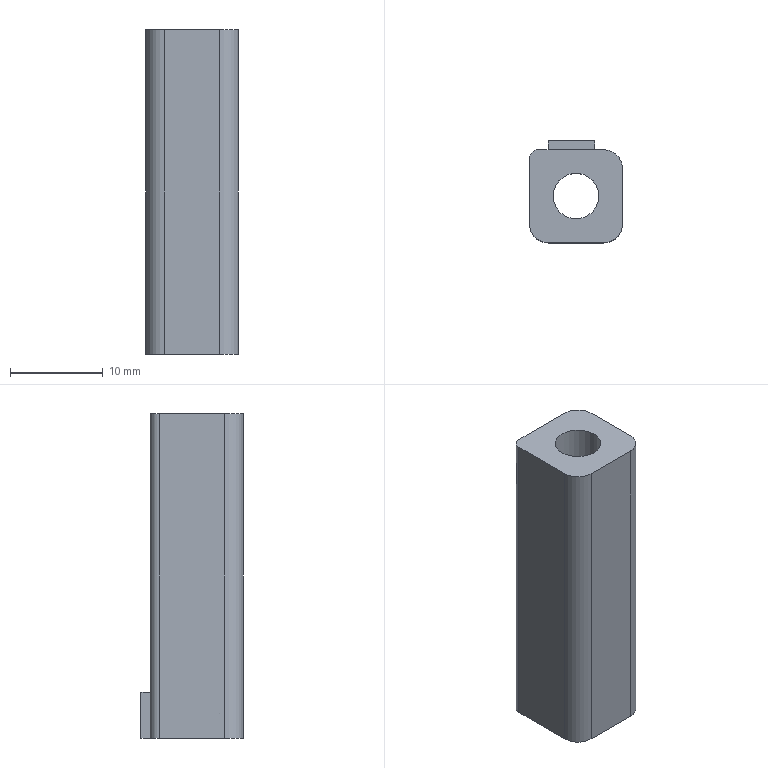Part | NX | features DIE-91 2 | 1 solid | 17 faces | box 10 x 11 x 35 mm | volume 2507 mm3 | plane 11 | cylinder 6 | commonest cylinder face diameters 4 x3 2 x1 4.92 x1 5.92 x1
STEP:
#1=CARTESIAN_POINT('',(4108.236,-844.622,828.716));
#2=VERTEX_POINT('',#1);
#3=CARTESIAN_POINT('',(4113.236,-844.622,828.716));
#4=VERTEX_POINT('',#3);
#5=CARTESIAN_POINT('',(4111.236,-844.622,828.716));
#6=DIRECTION('',(1.,0.,0.));
#7=VECTOR('',#6,1000.);
#8=LINE('',#5,#7);
#9=EDGE_CURVE('',#2,#4,#8,.T.);
#10=ORIENTED_EDGE('',*,*,#9,.F.);
#11=CARTESIAN_POINT('',(4108.236,-844.622,823.716));
#12=VERTEX_POINT('',#11);
#13=CARTESIAN_POINT('',(4108.236,-844.622,823.716));
#14=DIRECTION('',(0.,0.,-1.));
#15=VECTOR('',#14,1000.);
#16=LINE('',#13,#15);
#17=EDGE_CURVE('',#2,#12,#16,.T.);
#18=ORIENTED_EDGE('',*,*,#17,.T.);
#19=CARTESIAN_POINT('',(4107.236,-844.622,823.716));
#20=VERTEX_POINT('',#19);
#21=CARTESIAN_POINT('',(4111.236,-844.622,823.716));
#22=DIRECTION('',(-1.,0.,0.));
#23=VECTOR('',#22,1000.);
#24=LINE('',#21,#23);
#25=EDGE_CURVE('',#20,#12,#24,.F.);
#26=ORIENTED_EDGE('',*,*,#25,.F.);
#27=CARTESIAN_POINT('',(4107.236,-844.622,858.716));
#28=VERTEX_POINT('',#27);
#29=CARTESIAN_POINT('',(4107.236,-844.622,823.716));
#30=DIRECTION('',(0.,0.,1.));
#31=VECTOR('',#30,1000.);
#32=LINE('',#29,#31);
#33=EDGE_CURVE('',#20,#28,#32,.T.);
#34=ORIENTED_EDGE('',*,*,#33,.T.);
#35=CARTESIAN_POINT('',(4114.236,-844.622,858.716));
#36=VERTEX_POINT('',#35);
#37=CARTESIAN_POINT('',(4111.236,-844.622,858.716));
#38=DIRECTION('',(1.,0.,0.));
#39=VECTOR('',#38,1000.);
#40=LINE('',#37,#39);
#41=EDGE_CURVE('',#28,#36,#40,.T.);
#42=ORIENTED_EDGE('',*,*,#41,.T.);
#43=CARTESIAN_POINT('',(4114.236,-844.622,823.716));
#44=VERTEX_POINT('',#43);
#45=CARTESIAN_POINT('',(4114.236,-844.622,823.716));
#46=DIRECTION('',(0.,0.,1.));
#47=VECTOR('',#46,1000.);
#48=LINE('',#45,#47);
#49=EDGE_CURVE('',#36,#44,#48,.F.);
#50=ORIENTED_EDGE('',*,*,#49,.T.);
#51=CARTESIAN_POINT('',(4113.236,-844.622,823.716));
#52=VERTEX_POINT('',#51);
#53=CARTESIAN_POINT('',(4111.236,-844.622,823.716));
#54=DIRECTION('',(-1.,0.,0.));
#55=VECTOR('',#54,1000.);
#56=LINE('',#53,#55);
#57=EDGE_CURVE('',#52,#44,#56,.F.);
#58=ORIENTED_EDGE('',*,*,#57,.F.);
#59=CARTESIAN_POINT('',(4113.236,-844.622,823.716));
#60=DIRECTION('',(0.,0.,1.));
#61=VECTOR('',#60,1000.);
#62=LINE('',#59,#61);
#63=EDGE_CURVE('',#52,#4,#62,.T.);
#64=ORIENTED_EDGE('',*,*,#63,.T.);
#65=EDGE_LOOP('',(#10,#18,#26,#34,#42,#50,#58,#64));
#66=FACE_BOUND('',#65,.T.);
#67=CARTESIAN_POINT('',(4111.236,-844.622,823.716));
#68=DIRECTION('',(0.,1.,0.));
#69=DIRECTION('',(0.,0.,1.));
#70=AXIS2_PLACEMENT_3D('',#67,#68,#69);
#71=PLANE('',#70);
#72=ADVANCED_FACE('',(#66),#71,.T.);
#73=CARTESIAN_POINT('',(4108.276,-849.622,823.716));
#74=VERTEX_POINT('',#73);
#75=CARTESIAN_POINT('',(4111.236,-849.622,823.716));
#76=DIRECTION('',(0.,0.,-1.));
#77=DIRECTION('',(-1.,0.,0.));
#78=AXIS2_PLACEMENT_3D('',#75,#76,#77);
#79=CIRCLE('',#78,2.96);
#80=EDGE_CURVE('',#74,#74,#79,.T.);
#81=ORIENTED_EDGE('',*,*,#80,.T.);
#82=CARTESIAN_POINT('',(4108.276,-849.622,853.716));
#83=VERTEX_POINT('',#82);
#84=CARTESIAN_POINT('',(4108.276,-849.622,862.216));
#85=DIRECTION('',(0.,0.,-1.));
#86=VECTOR('',#85,1000.);
#87=LINE('',#84,#86);
#88=EDGE_CURVE('',#83,#74,#87,.T.);
#89=ORIENTED_EDGE('',*,*,#88,.F.);
#90=CARTESIAN_POINT('',(4111.236,-849.622,853.716));
#91=DIRECTION('',(0.,0.,1.));
#92=DIRECTION('',(1.,0.,0.));
#93=AXIS2_PLACEMENT_3D('',#90,#91,#92);
#94=CIRCLE('',#93,2.96);
#95=EDGE_CURVE('',#83,#83,#94,.F.);
#96=ORIENTED_EDGE('',*,*,#95,.F.);
#97=ORIENTED_EDGE('',*,*,#88,.T.);
#98=EDGE_LOOP('',(#81,#89,#96,#97));
#99=FACE_BOUND('',#98,.T.);
#100=CARTESIAN_POINT('',(4111.236,-849.622,862.216));
#101=DIRECTION('',(0.,0.,-1.));
#102=DIRECTION('',(-1.,0.,0.));
#103=AXIS2_PLACEMENT_3D('',#100,#101,#102);
#104=CYLINDRICAL_SURFACE('',#103,2.96);
#105=ADVANCED_FACE('',(#99),#104,.F.);
#106=ORIENTED_EDGE('',*,*,#25,.T.);
#107=CARTESIAN_POINT('',(4108.236,-843.622,823.716));
#108=VERTEX_POINT('',#107);
#109=CARTESIAN_POINT('',(4108.236,-843.622,823.716));
#110=DIRECTION('',(0.,-1.,0.));
#111=VECTOR('',#110,1000.);
#112=LINE('',#109,#111);
#113=EDGE_CURVE('',#108,#12,#112,.T.);
#114=ORIENTED_EDGE('',*,*,#113,.F.);
#115=CARTESIAN_POINT('',(4113.236,-843.622,823.716));
#116=VERTEX_POINT('',#115);
#117=CARTESIAN_POINT('',(4114.236,-843.622,823.716));
#118=DIRECTION('',(-1.,0.,0.));
#119=VECTOR('',#118,1000.);
#120=LINE('',#117,#119);
#121=EDGE_CURVE('',#116,#108,#120,.T.);
#122=ORIENTED_EDGE('',*,*,#121,.F.);
#123=CARTESIAN_POINT('',(4113.236,-844.672,823.716));
#124=DIRECTION('',(0.,1.,0.));
#125=VECTOR('',#124,1000.);
#126=LINE('',#123,#125);
#127=EDGE_CURVE('',#52,#116,#126,.T.);
#128=ORIENTED_EDGE('',*,*,#127,.F.);
#129=ORIENTED_EDGE('',*,*,#57,.T.);
#130=CARTESIAN_POINT('',(4116.236,-846.622,823.716));
#131=VERTEX_POINT('',#130);
#132=CARTESIAN_POINT('',(4114.236,-846.622,823.716));
#133=DIRECTION('',(0.,0.,-1.));
#134=DIRECTION('',(-1.,0.,0.));
#135=AXIS2_PLACEMENT_3D('',#132,#133,#134);
#136=CIRCLE('',#135,2.);
#137=EDGE_CURVE('',#131,#44,#136,.F.);
#138=ORIENTED_EDGE('',*,*,#137,.F.);
#139=CARTESIAN_POINT('',(4116.236,-852.622,823.716));
#140=VERTEX_POINT('',#139);
#141=CARTESIAN_POINT('',(4116.236,-849.622,823.716));
#142=DIRECTION('',(0.,1.,0.));
#143=VECTOR('',#142,1000.);
#144=LINE('',#141,#143);
#145=EDGE_CURVE('',#140,#131,#144,.T.);
#146=ORIENTED_EDGE('',*,*,#145,.F.);
#147=CARTESIAN_POINT('',(4114.236,-854.622,823.716));
#148=VERTEX_POINT('',#147);
#149=CARTESIAN_POINT('',(4114.236,-852.622,823.716));
#150=DIRECTION('',(0.,0.,-1.));
#151=DIRECTION('',(-1.,0.,0.));
#152=AXIS2_PLACEMENT_3D('',#149,#150,#151);
#153=CIRCLE('',#152,2.);
#154=EDGE_CURVE('',#140,#148,#153,.T.);
#155=ORIENTED_EDGE('',*,*,#154,.T.);
#156=CARTESIAN_POINT('',(4108.236,-854.622,823.716));
#157=VERTEX_POINT('',#156);
#158=CARTESIAN_POINT('',(4111.236,-854.622,823.716));
#159=DIRECTION('',(1.,0.,0.));
#160=VECTOR('',#159,1000.);
#161=LINE('',#158,#160);
#162=EDGE_CURVE('',#157,#148,#161,.T.);
#163=ORIENTED_EDGE('',*,*,#162,.F.);
#164=CARTESIAN_POINT('',(4106.236,-852.622,823.716));
#165=VERTEX_POINT('',#164);
#166=CARTESIAN_POINT('',(4108.236,-852.622,823.716));
#167=DIRECTION('',(0.,0.,-1.));
#168=DIRECTION('',(-1.,0.,0.));
#169=AXIS2_PLACEMENT_3D('',#166,#167,#168);
#170=CIRCLE('',#169,2.);
#171=EDGE_CURVE('',#157,#165,#170,.T.);
#172=ORIENTED_EDGE('',*,*,#171,.T.);
#173=CARTESIAN_POINT('',(4106.236,-845.622,823.716));
#174=VERTEX_POINT('',#173);
#175=CARTESIAN_POINT('',(4106.236,-849.622,823.716));
#176=DIRECTION('',(0.,-1.,0.));
#177=VECTOR('',#176,1000.);
#178=LINE('',#175,#177);
#179=EDGE_CURVE('',#165,#174,#178,.F.);
#180=ORIENTED_EDGE('',*,*,#179,.T.);
#181=CARTESIAN_POINT('',(4107.236,-845.622,823.716));
#182=DIRECTION('',(0.,0.,-1.));
#183=DIRECTION('',(-1.,0.,0.));
#184=AXIS2_PLACEMENT_3D('',#181,#182,#183);
#185=CIRCLE('',#184,1.);
#186=EDGE_CURVE('',#174,#20,#185,.T.);
#187=ORIENTED_EDGE('',*,*,#186,.T.);
#188=EDGE_LOOP('',(#106,#114,#122,#128,#129,#138,#146,#155,#163,#172,#180,#187));
#189=FACE_BOUND('',#188,.T.);
#190=ORIENTED_EDGE('',*,*,#80,.F.);
#191=EDGE_LOOP('',(#190));
#192=FACE_BOUND('',#191,.T.);
#193=CARTESIAN_POINT('',(4123.586,-858.122,823.716));
#194=DIRECTION('',(0.,0.,-1.));
#195=DIRECTION('',(-1.,0.,0.));
#196=AXIS2_PLACEMENT_3D('',#193,#194,#195);
#197=PLANE('',#196);
#198=ADVANCED_FACE('',(#189,#192),#197,.T.);
#199=CARTESIAN_POINT('',(4108.776,-849.622,853.716));
#200=VERTEX_POINT('',#199);
#201=CARTESIAN_POINT('',(4111.236,-849.622,853.716));
#202=DIRECTION('',(0.,0.,1.));
#203=DIRECTION('',(1.,0.,0.));
#204=AXIS2_PLACEMENT_3D('',#201,#202,#203);
#205=CIRCLE('',#204,2.46);
#206=EDGE_CURVE('',#200,#200,#205,.T.);
#207=ORIENTED_EDGE('',*,*,#206,.T.);
#208=EDGE_LOOP('',(#207));
#209=FACE_BOUND('',#208,.T.);
#210=ORIENTED_EDGE('',*,*,#95,.T.);
#211=EDGE_LOOP('',(#210));
#212=FACE_BOUND('',#211,.T.);
#213=CARTESIAN_POINT('',(4079.736,-858.122,853.716));
#214=DIRECTION('',(0.,0.,1.));
#215=DIRECTION('',(1.,0.,0.));
#216=AXIS2_PLACEMENT_3D('',#213,#214,#215);
#217=PLANE('',#216);
#218=ADVANCED_FACE('',(#209,#212),#217,.F.);
#219=CARTESIAN_POINT('',(4108.776,-849.622,858.716));
#220=VERTEX_POINT('',#219);
#221=CARTESIAN_POINT('',(4108.776,-849.622,862.216));
#222=DIRECTION('',(0.,0.,-1.));
#223=VECTOR('',#222,1000.);
#224=LINE('',#221,#223);
#225=EDGE_CURVE('',#220,#200,#224,.T.);
#226=ORIENTED_EDGE('',*,*,#225,.T.);
#227=ORIENTED_EDGE('',*,*,#206,.F.);
#228=ORIENTED_EDGE('',*,*,#225,.F.);
#229=CARTESIAN_POINT('',(4111.236,-849.622,858.716));
#230=DIRECTION('',(0.,0.,1.));
#231=DIRECTION('',(1.,0.,0.));
#232=AXIS2_PLACEMENT_3D('',#229,#230,#231);
#233=CIRCLE('',#232,2.46);
#234=EDGE_CURVE('',#220,#220,#233,.T.);
#235=ORIENTED_EDGE('',*,*,#234,.T.);
#236=EDGE_LOOP('',(#226,#227,#228,#235));
#237=FACE_BOUND('',#236,.T.);
#238=CARTESIAN_POINT('',(4111.236,-849.622,862.216));
#239=DIRECTION('',(0.,0.,-1.));
#240=DIRECTION('',(-1.,0.,0.));
#241=AXIS2_PLACEMENT_3D('',#238,#239,#240);
#242=CYLINDRICAL_SURFACE('',#241,2.46);
#243=ADVANCED_FACE('',(#237),#242,.F.);
#244=ORIENTED_EDGE('',*,*,#234,.F.);
#245=EDGE_LOOP('',(#244));
#246=FACE_BOUND('',#245,.T.);
#247=CARTESIAN_POINT('',(4106.236,-852.622,858.716));
#248=VERTEX_POINT('',#247);
#249=CARTESIAN_POINT('',(4106.236,-845.622,858.716));
#250=VERTEX_POINT('',#249);
#251=CARTESIAN_POINT('',(4106.236,-849.622,858.716));
#252=DIRECTION('',(0.,1.,0.));
#253=VECTOR('',#252,1000.);
#254=LINE('',#251,#253);
#255=EDGE_CURVE('',#248,#250,#254,.T.);
#256=ORIENTED_EDGE('',*,*,#255,.F.);
#257=CARTESIAN_POINT('',(4108.236,-854.622,858.716));
#258=VERTEX_POINT('',#257);
#259=CARTESIAN_POINT('',(4108.236,-852.622,858.716));
#260=DIRECTION('',(0.,0.,1.));
#261=DIRECTION('',(1.,0.,0.));
#262=AXIS2_PLACEMENT_3D('',#259,#260,#261);
#263=CIRCLE('',#262,2.);
#264=EDGE_CURVE('',#258,#248,#263,.F.);
#265=ORIENTED_EDGE('',*,*,#264,.F.);
#266=CARTESIAN_POINT('',(4114.236,-854.622,858.716));
#267=VERTEX_POINT('',#266);
#268=CARTESIAN_POINT('',(4111.236,-854.622,858.716));
#269=DIRECTION('',(-1.,0.,0.));
#270=VECTOR('',#269,1000.);
#271=LINE('',#268,#270);
#272=EDGE_CURVE('',#258,#267,#271,.F.);
#273=ORIENTED_EDGE('',*,*,#272,.T.);
#274=CARTESIAN_POINT('',(4116.236,-852.622,858.716));
#275=VERTEX_POINT('',#274);
#276=CARTESIAN_POINT('',(4114.236,-852.622,858.716));
#277=DIRECTION('',(0.,0.,1.));
#278=DIRECTION('',(1.,0.,0.));
#279=AXIS2_PLACEMENT_3D('',#276,#277,#278);
#280=CIRCLE('',#279,2.);
#281=EDGE_CURVE('',#275,#267,#280,.F.);
#282=ORIENTED_EDGE('',*,*,#281,.F.);
#283=CARTESIAN_POINT('',(4116.236,-846.622,858.716));
#284=VERTEX_POINT('',#283);
#285=CARTESIAN_POINT('',(4116.236,-849.622,858.716));
#286=DIRECTION('',(0.,-1.,0.));
#287=VECTOR('',#286,1000.);
#288=LINE('',#285,#287);
#289=EDGE_CURVE('',#275,#284,#288,.F.);
#290=ORIENTED_EDGE('',*,*,#289,.T.);
#291=CARTESIAN_POINT('',(4114.236,-846.622,858.716));
#292=DIRECTION('',(0.,0.,1.));
#293=DIRECTION('',(1.,0.,0.));
#294=AXIS2_PLACEMENT_3D('',#291,#292,#293);
#295=CIRCLE('',#294,2.);
#296=EDGE_CURVE('',#284,#36,#295,.T.);
#297=ORIENTED_EDGE('',*,*,#296,.T.);
#298=ORIENTED_EDGE('',*,*,#41,.F.);
#299=CARTESIAN_POINT('',(4107.236,-845.622,858.716));
#300=DIRECTION('',(0.,0.,1.));
#301=DIRECTION('',(1.,0.,0.));
#302=AXIS2_PLACEMENT_3D('',#299,#300,#301);
#303=CIRCLE('',#302,1.);
#304=EDGE_CURVE('',#28,#250,#303,.T.);
#305=ORIENTED_EDGE('',*,*,#304,.T.);
#306=EDGE_LOOP('',(#256,#265,#273,#282,#290,#297,#298,#305));
#307=FACE_BOUND('',#306,.T.);
#308=CARTESIAN_POINT('',(4123.586,-858.122,858.716));
#309=DIRECTION('',(0.,0.,1.));
#310=DIRECTION('',(-1.,0.,0.));
#311=AXIS2_PLACEMENT_3D('',#308,#309,#310);
#312=PLANE('',#311);
#313=ADVANCED_FACE('',(#246,#307),#312,.T.);
#314=ORIENTED_EDGE('',*,*,#186,.F.);
#315=CARTESIAN_POINT('',(4106.236,-845.622,823.716));
#316=DIRECTION('',(0.,0.,1.));
#317=VECTOR('',#316,1000.);
#318=LINE('',#315,#317);
#319=EDGE_CURVE('',#250,#174,#318,.F.);
#320=ORIENTED_EDGE('',*,*,#319,.F.);
#321=ORIENTED_EDGE('',*,*,#304,.F.);
#322=ORIENTED_EDGE('',*,*,#33,.F.);
#323=EDGE_LOOP('',(#314,#320,#321,#322));
#324=FACE_BOUND('',#323,.T.);
#325=CARTESIAN_POINT('',(4107.236,-845.622,823.716));
#326=DIRECTION('',(0.,0.,1.));
#327=DIRECTION('',(1.,0.,0.));
#328=AXIS2_PLACEMENT_3D('',#325,#326,#327);
#329=CYLINDRICAL_SURFACE('',#328,1.);
#330=ADVANCED_FACE('',(#324),#329,.T.);
#331=ORIENTED_EDGE('',*,*,#171,.F.);
#332=CARTESIAN_POINT('',(4108.236,-854.622,823.716));
#333=DIRECTION('',(0.,0.,1.));
#334=VECTOR('',#333,1000.);
#335=LINE('',#332,#334);
#336=EDGE_CURVE('',#258,#157,#335,.F.);
#337=ORIENTED_EDGE('',*,*,#336,.F.);
#338=ORIENTED_EDGE('',*,*,#264,.T.);
#339=CARTESIAN_POINT('',(4106.236,-852.622,823.716));
#340=DIRECTION('',(0.,0.,1.));
#341=VECTOR('',#340,1000.);
#342=LINE('',#339,#341);
#343=EDGE_CURVE('',#165,#248,#342,.T.);
#344=ORIENTED_EDGE('',*,*,#343,.F.);
#345=EDGE_LOOP('',(#331,#337,#338,#344));
#346=FACE_BOUND('',#345,.T.);
#347=CARTESIAN_POINT('',(4108.236,-852.622,823.716));
#348=DIRECTION('',(0.,0.,1.));
#349=DIRECTION('',(1.,0.,0.));
#350=AXIS2_PLACEMENT_3D('',#347,#348,#349);
#351=CYLINDRICAL_SURFACE('',#350,2.);
#352=ADVANCED_FACE('',(#346),#351,.T.);
#353=ORIENTED_EDGE('',*,*,#154,.F.);
#354=CARTESIAN_POINT('',(4116.236,-852.622,823.716));
#355=DIRECTION('',(0.,0.,1.));
#356=VECTOR('',#355,1000.);
#357=LINE('',#354,#356);
#358=EDGE_CURVE('',#275,#140,#357,.F.);
#359=ORIENTED_EDGE('',*,*,#358,.F.);
#360=ORIENTED_EDGE('',*,*,#281,.T.);
#361=CARTESIAN_POINT('',(4114.236,-854.622,823.716));
#362=DIRECTION('',(0.,0.,1.));
#363=VECTOR('',#362,1000.);
#364=LINE('',#361,#363);
#365=EDGE_CURVE('',#148,#267,#364,.T.);
#366=ORIENTED_EDGE('',*,*,#365,.F.);
#367=EDGE_LOOP('',(#353,#359,#360,#366));
#368=FACE_BOUND('',#367,.T.);
#369=CARTESIAN_POINT('',(4114.236,-852.622,823.716));
#370=DIRECTION('',(0.,0.,1.));
#371=DIRECTION('',(1.,0.,0.));
#372=AXIS2_PLACEMENT_3D('',#369,#370,#371);
#373=CYLINDRICAL_SURFACE('',#372,2.);
#374=ADVANCED_FACE('',(#368),#373,.T.);
#375=ORIENTED_EDGE('',*,*,#137,.T.);
#376=ORIENTED_EDGE('',*,*,#49,.F.);
#377=ORIENTED_EDGE('',*,*,#296,.F.);
#378=CARTESIAN_POINT('',(4116.236,-846.622,823.716));
#379=DIRECTION('',(0.,0.,1.));
#380=VECTOR('',#379,1000.);
#381=LINE('',#378,#380);
#382=EDGE_CURVE('',#131,#284,#381,.T.);
#383=ORIENTED_EDGE('',*,*,#382,.F.);
#384=EDGE_LOOP('',(#375,#376,#377,#383));
#385=FACE_BOUND('',#384,.T.);
#386=CARTESIAN_POINT('',(4114.236,-846.622,823.716));
#387=DIRECTION('',(0.,0.,1.));
#388=DIRECTION('',(1.,0.,0.));
#389=AXIS2_PLACEMENT_3D('',#386,#387,#388);
#390=CYLINDRICAL_SURFACE('',#389,2.);
#391=ADVANCED_FACE('',(#385),#390,.T.);
#392=ORIENTED_EDGE('',*,*,#145,.T.);
#393=ORIENTED_EDGE('',*,*,#382,.T.);
#394=ORIENTED_EDGE('',*,*,#289,.F.);
#395=ORIENTED_EDGE('',*,*,#358,.T.);
#396=EDGE_LOOP('',(#392,#393,#394,#395));
#397=FACE_BOUND('',#396,.T.);
#398=CARTESIAN_POINT('',(4116.236,-849.622,823.716));
#399=DIRECTION('',(1.,0.,0.));
#400=DIRECTION('',(0.,0.,-1.));
#401=AXIS2_PLACEMENT_3D('',#398,#399,#400);
#402=PLANE('',#401);
#403=ADVANCED_FACE('',(#397),#402,.T.);
#404=ORIENTED_EDGE('',*,*,#255,.T.);
#405=ORIENTED_EDGE('',*,*,#319,.T.);
#406=ORIENTED_EDGE('',*,*,#179,.F.);
#407=ORIENTED_EDGE('',*,*,#343,.T.);
#408=EDGE_LOOP('',(#404,#405,#406,#407));
#409=FACE_BOUND('',#408,.T.);
#410=CARTESIAN_POINT('',(4106.236,-849.622,823.716));
#411=DIRECTION('',(-1.,0.,0.));
#412=DIRECTION('',(0.,0.,1.));
#413=AXIS2_PLACEMENT_3D('',#410,#411,#412);
#414=PLANE('',#413);
#415=ADVANCED_FACE('',(#409),#414,.T.);
#416=ORIENTED_EDGE('',*,*,#162,.T.);
#417=ORIENTED_EDGE('',*,*,#365,.T.);
#418=ORIENTED_EDGE('',*,*,#272,.F.);
#419=ORIENTED_EDGE('',*,*,#336,.T.);
#420=EDGE_LOOP('',(#416,#417,#418,#419));
#421=FACE_BOUND('',#420,.T.);
#422=CARTESIAN_POINT('',(4111.236,-854.622,823.716));
#423=DIRECTION('',(0.,-1.,0.));
#424=DIRECTION('',(0.,0.,-1.));
#425=AXIS2_PLACEMENT_3D('',#422,#423,#424);
#426=PLANE('',#425);
#427=ADVANCED_FACE('',(#421),#426,.T.);
#428=ORIENTED_EDGE('',*,*,#17,.F.);
#429=CARTESIAN_POINT('',(4108.236,-843.622,828.716));
#430=VERTEX_POINT('',#429);
#431=CARTESIAN_POINT('',(4108.236,-843.622,828.716));
#432=DIRECTION('',(0.,-1.,0.));
#433=VECTOR('',#432,1000.);
#434=LINE('',#431,#433);
#435=EDGE_CURVE('',#430,#2,#434,.T.);
#436=ORIENTED_EDGE('',*,*,#435,.F.);
#437=CARTESIAN_POINT('',(4108.236,-843.622,828.716));
#438=DIRECTION('',(0.,0.,-1.));
#439=VECTOR('',#438,1000.);
#440=LINE('',#437,#439);
#441=EDGE_CURVE('',#430,#108,#440,.T.);
#442=ORIENTED_EDGE('',*,*,#441,.T.);
#443=ORIENTED_EDGE('',*,*,#113,.T.);
#444=EDGE_LOOP('',(#428,#436,#442,#443));
#445=FACE_BOUND('',#444,.T.);
#446=CARTESIAN_POINT('',(4108.236,-843.622,828.716));
#447=DIRECTION('',(1.,0.,0.));
#448=DIRECTION('',(0.,0.,-1.));
#449=AXIS2_PLACEMENT_3D('',#446,#447,#448);
#450=PLANE('',#449);
#451=ADVANCED_FACE('',(#445),#450,.F.);
#452=ORIENTED_EDGE('',*,*,#63,.F.);
#453=ORIENTED_EDGE('',*,*,#127,.T.);
#454=CARTESIAN_POINT('',(4113.236,-843.622,828.716));
#455=VERTEX_POINT('',#454);
#456=CARTESIAN_POINT('',(4113.236,-843.622,828.716));
#457=DIRECTION('',(0.,0.,-1.));
#458=VECTOR('',#457,1000.);
#459=LINE('',#456,#458);
#460=EDGE_CURVE('',#455,#116,#459,.T.);
#461=ORIENTED_EDGE('',*,*,#460,.F.);
#462=CARTESIAN_POINT('',(4113.236,-844.672,828.716));
#463=DIRECTION('',(0.,1.,0.));
#464=VECTOR('',#463,1000.);
#465=LINE('',#462,#464);
#466=EDGE_CURVE('',#4,#455,#465,.T.);
#467=ORIENTED_EDGE('',*,*,#466,.F.);
#468=EDGE_LOOP('',(#452,#453,#461,#467));
#469=FACE_BOUND('',#468,.T.);
#470=CARTESIAN_POINT('',(4113.236,-844.672,828.716));
#471=DIRECTION('',(-1.,0.,0.));
#472=DIRECTION('',(0.,0.,1.));
#473=AXIS2_PLACEMENT_3D('',#470,#471,#472);
#474=PLANE('',#473);
#475=ADVANCED_FACE('',(#469),#474,.F.);
#476=ORIENTED_EDGE('',*,*,#121,.T.);
#477=ORIENTED_EDGE('',*,*,#441,.F.);
#478=CARTESIAN_POINT('',(4114.236,-843.622,828.716));
#479=DIRECTION('',(-1.,0.,0.));
#480=VECTOR('',#479,1000.);
#481=LINE('',#478,#480);
#482=EDGE_CURVE('',#455,#430,#481,.T.);
#483=ORIENTED_EDGE('',*,*,#482,.F.);
#484=ORIENTED_EDGE('',*,*,#460,.T.);
#485=EDGE_LOOP('',(#476,#477,#483,#484));
#486=FACE_BOUND('',#485,.T.);
#487=CARTESIAN_POINT('',(4114.236,-843.622,828.716));
#488=DIRECTION('',(0.,-1.,0.));
#489=DIRECTION('',(0.,0.,-1.));
#490=AXIS2_PLACEMENT_3D('',#487,#488,#489);
#491=PLANE('',#490);
#492=ADVANCED_FACE('',(#486),#491,.F.);
#493=ORIENTED_EDGE('',*,*,#435,.T.);
#494=ORIENTED_EDGE('',*,*,#9,.T.);
#495=ORIENTED_EDGE('',*,*,#466,.T.);
#496=ORIENTED_EDGE('',*,*,#482,.T.);
#497=EDGE_LOOP('',(#493,#494,#495,#496));
#498=FACE_BOUND('',#497,.T.);
#499=CARTESIAN_POINT('',(0.,0.,828.716));
#500=DIRECTION('',(0.,0.,1.));
#501=DIRECTION('',(1.,0.,0.));
#502=AXIS2_PLACEMENT_3D('',#499,#500,#501);
#503=PLANE('',#502);
#504=ADVANCED_FACE('',(#498),#503,.T.);
#505=CLOSED_SHELL('',(#72,#105,#198,#218,#243,#313,#330,#352,#374,#391,#403,#415,#427,#451,#475,#492,#504));
#506=MANIFOLD_SOLID_BREP('',#505);
#507=(LENGTH_UNIT()NAMED_UNIT(*)SI_UNIT(.MILLI.,.METRE.));
#508=UNCERTAINTY_MEASURE_WITH_UNIT(LENGTH_MEASURE(0.00001),#507,'','');
#509=(NAMED_UNIT(*)PLANE_ANGLE_UNIT()SI_UNIT($,.RADIAN.));
#510=(NAMED_UNIT(*)SI_UNIT($,.STERADIAN.)SOLID_ANGLE_UNIT());
#511=(GEOMETRIC_REPRESENTATION_CONTEXT(3)GLOBAL_UNCERTAINTY_ASSIGNED_CONTEXT((#508))GLOBAL_UNIT_ASSIGNED_CONTEXT((#507,#509,#510))REPRESENTATION_CONTEXT('',''));
#512=ADVANCED_BREP_SHAPE_REPRESENTATION('',(#506),#511);